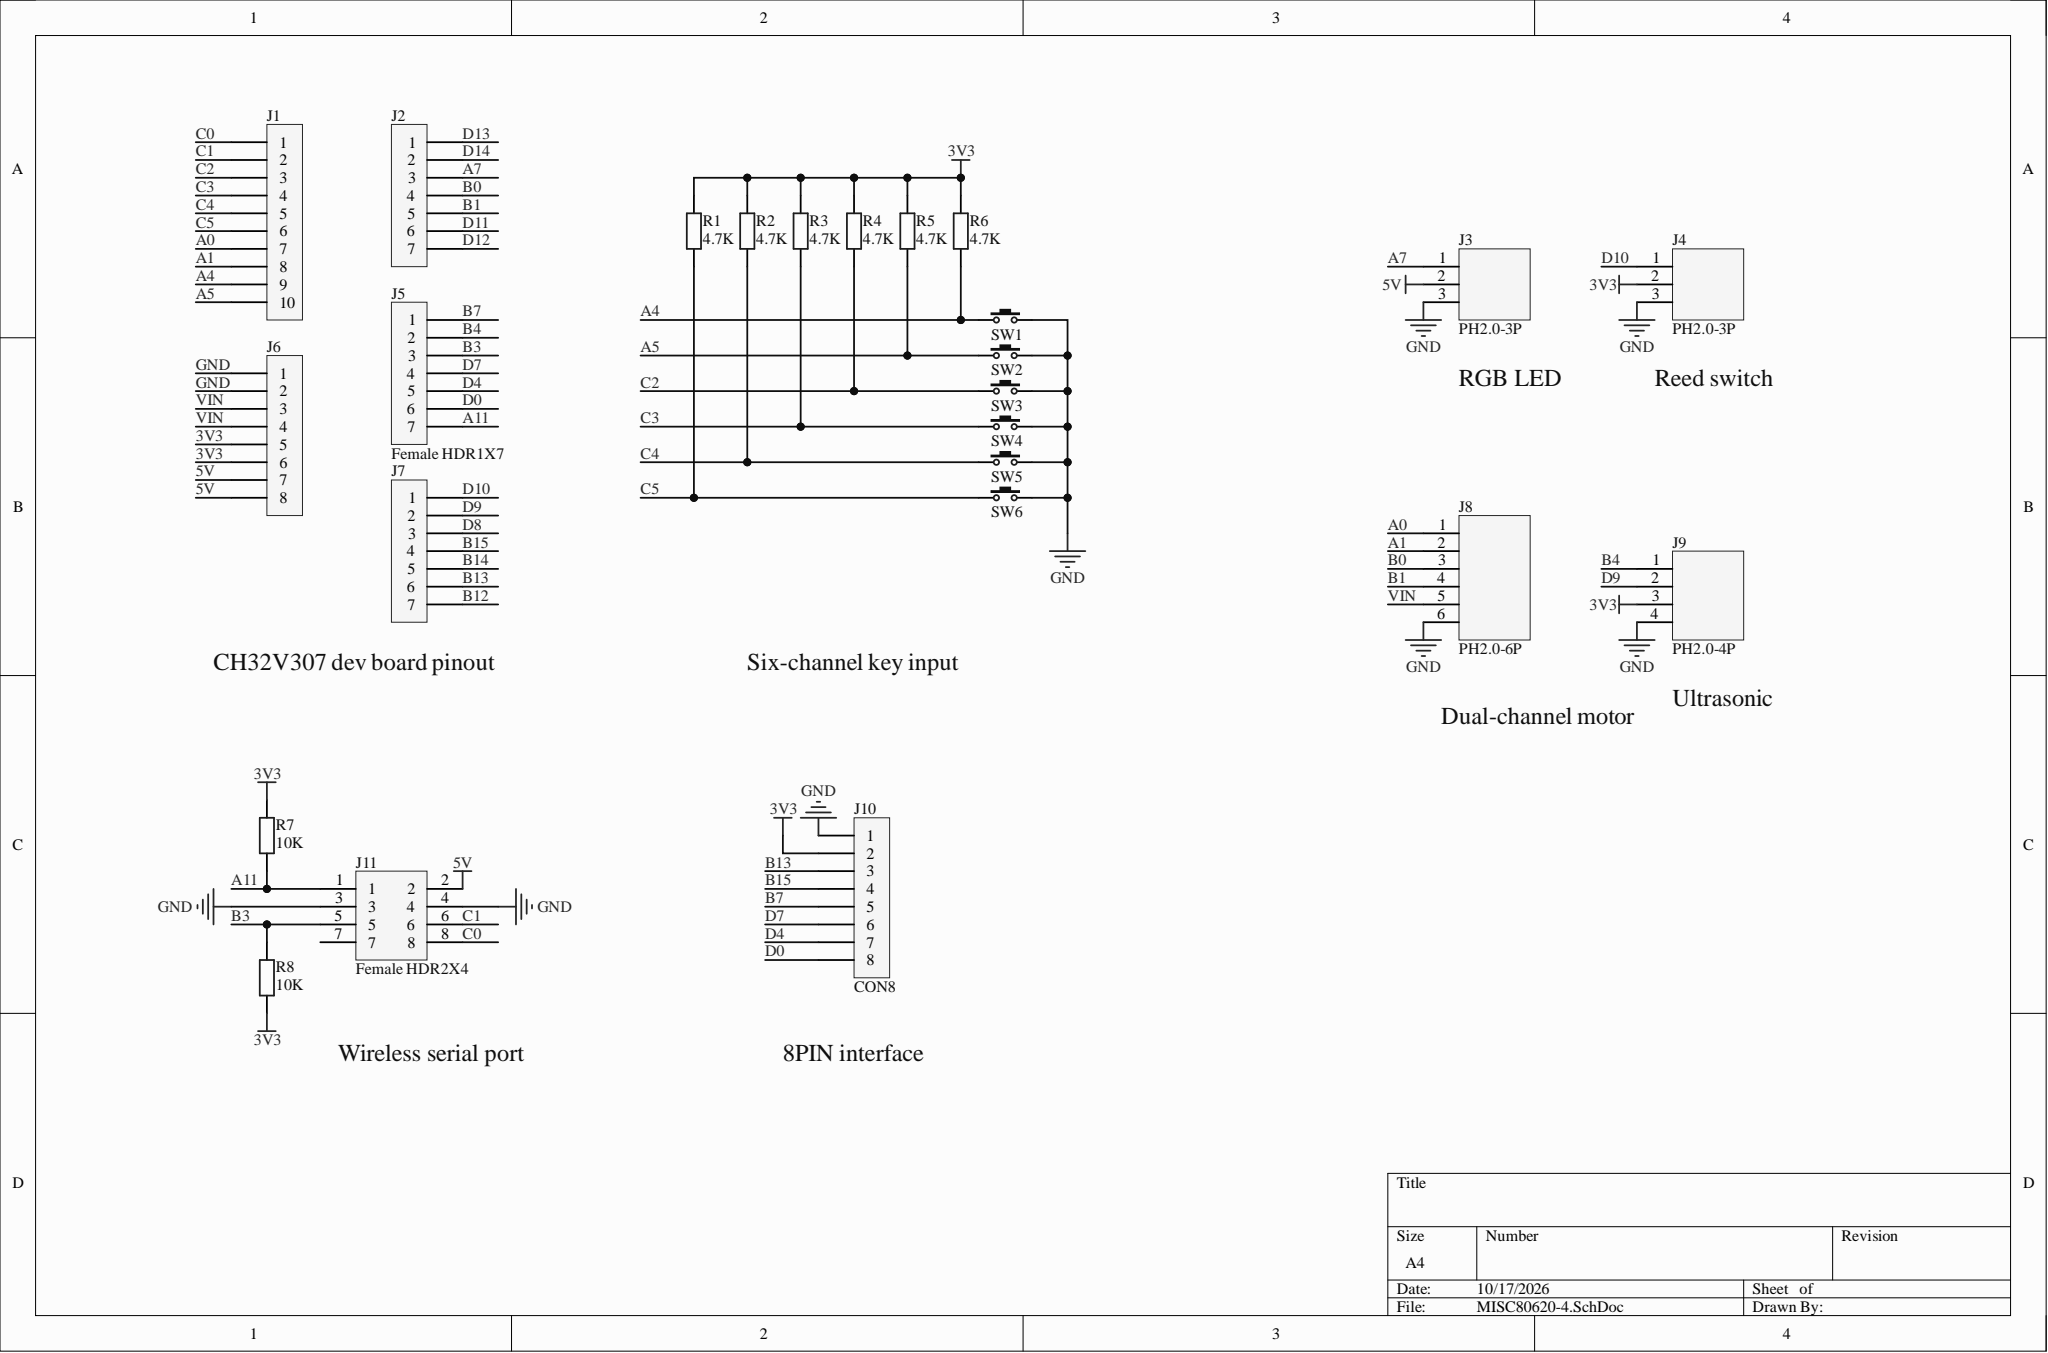Circuit board | Altium Designer | 25 parts | 28 nets
Bill of materials:
Comment,Description,Designator,Footprint,LibRef,Quantity
"Female HDR1X10","","J1","Fe-HDR1X10/2.54-S","Female HDR1X10","1"
"Female HDR1X7","","J2, J5, J7","Fe-HDR1X7/2.54-S","Female HDR1X7","3"
"PH2.0-3P","","J3, J4","PH2.0-3P","PH2.0-3P","2"
"Female HDR1X8","","J6","Fe-HDR1X8/2.54-S","Female HDR1X8","1"
"PH2.0-6P","","J8","PH2.0-6P","PH2.0-6P","1"
"PH2.0-4P","","J9","PH2.0-4P","PH2.0-4P","1"
"CON8","","J10","Fe-HDR1X8/2.54-S","Female HDR1X8","1"
"Female HDR2X4","","J11","Fe-HDR2X4/2.54-S","Female HDR2X4","1"
"4.7K","SMD resistor","R1, R2, R3, R4, R5, R6","R 0805_L","R","6"
"10K","SMD resistor","R7, R8","R 0805_L","R","2"
"3x6x5","3x6 tact switch","SW1, SW2, SW3, SW4, SW5, SW6","TSW DIP-3*6*4.3","TSW 3x6","6"
Netlist (Protel format):
[
J1
Fe-HDR1X10/2.54-S
Female HDR1X10



]
[
J2
Fe-HDR1X7/2.54-S
Female HDR1X7



]
[
J3
PH2.0-3P
PH2.0-3P



]
[
J4
PH2.0-3P
PH2.0-3P



]
[
J5
Fe-HDR1X7/2.54-S
Female HDR1X7



]
[
J6
Fe-HDR1X8/2.54-S
Female HDR1X8



]
[
J7
Fe-HDR1X7/2.54-S
Female HDR1X7



]
[
J8
PH2.0-6P
PH2.0-6P



]
[
J9
PH2.0-4P
PH2.0-4P



]
[
J10
Fe-HDR1X8/2.54-S
CON8



]
[
J11
Fe-HDR2X4/2.54-S
Female HDR2X4



]
[
R1
R 0805_L
4.7K



]
[
R2
R 0805_L
4.7K



]
[
R3
R 0805_L
4.7K



]
[
R4
R 0805_L
4.7K



]
[
R5
R 0805_L
4.7K



]
[
R6
R 0805_L
4.7K



]
[
R7
R 0805_L
10K



]
[
R8
R 0805_L
10K



]
[
SW1
TSW DIP-3*6*4.3
3x6x5



]
[
SW2
TSW DIP-3*6*4.3
3x6x5



]
[
SW3
TSW DIP-3*6*4.3
3x6x5



]
[
SW4
TSW DIP-3*6*4.3
3x6x5



]
[
SW5
TSW DIP-3*6*4.3
3x6x5



]
[
SW6
TSW DIP-3*6*4.3
3x6x5



]
(
VIN
J6-3
J6-4
J8-5
)
(
GND
J3-3
J4-3
J6-1
J6-2
J8-6
J9-4
J10-1
J11-3
J11-4
SW1-2
SW2-2
SW3-2
SW4-2
SW5-2
SW6-2
)
(
D10
J4-1
J7-1
)
(
D9
J7-2
J9-2
)
(
D7
J5-4
J10-6
)
(
D4
J5-5
J10-7
)
(
D0
J5-6
J10-8
)
(
C5
J1-6
R1-1
SW6-1
)
(
C4
J1-5
R2-1
SW5-1
)
(
C3
J1-4
R3-1
SW4-1
)
(
C2
J1-3
R4-1
SW3-1
)
(
C1
J1-2
J11-6
)
(
C0
J1-1
J11-8
)
(
B15
J7-4
J10-4
)
(
B13
J7-6
J10-3
)
(
B7
J5-1
J10-5
)
(
B4
J5-2
J9-1
)
(
B3
J5-3
J11-5
R8-2
)
(
B1
J2-5
J8-4
)
(
B0
J2-4
J8-3
)
(
A11
J5-7
J11-1
R7-1
)
(
A7
J2-3
J3-1
)
(
A5
J1-10
R5-1
SW2-1
)
(
A4
J1-9
R6-1
SW1-1
)
(
A1
J1-8
J8-2
)
(
A0
J1-7
J8-1
)
(
5V
J3-2
J6-7
J6-8
J11-2
)
(
3V3
J4-2
J6-5
J6-6
J9-3
J10-2
R1-2
R2-2
R3-2
R4-2
R5-2
R6-2
R7-2
R8-1
)